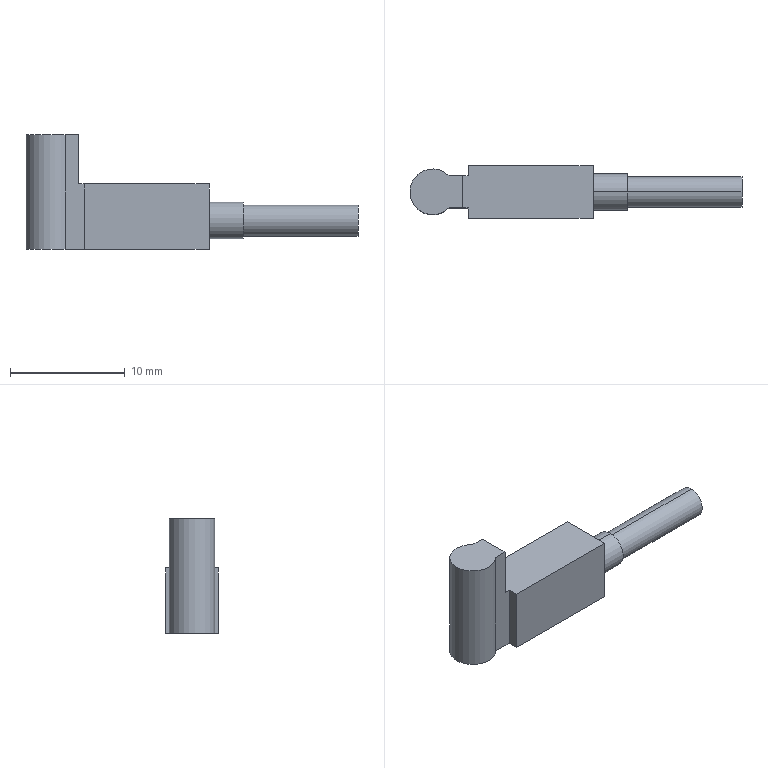Part | SolidWorks | features BaseBody 1 | 1 solid | 28 faces | box 29 x 4.6 x 10 mm | volume 522.344 mm3 | plane 18 | cylinder 10 | commonest cylinder face diameters 2.1 x3 2.5 x2 2.7 x2 3.2 x2 4 x1
STEP:
#1=CARTESIAN_POINT('',(27.,0.,-8.85));
#2=VERTEX_POINT('',#1);
#3=CARTESIAN_POINT('',(27.,0.,-6.15));
#4=VERTEX_POINT('',#3);
#5=CARTESIAN_POINT('',(27.,0.,-7.5));
#6=DIRECTION('',(1.,0.,0.));
#7=DIRECTION('',(0.,0.,-1.));
#8=AXIS2_PLACEMENT_3D('',#5,#6,#7);
#9=CIRCLE('',#8,1.35);
#10=EDGE_CURVE('',#2,#4,#9,.T.);
#11=ORIENTED_EDGE('',*,*,#10,.F.);
#12=CARTESIAN_POINT('',(17.,0.,-8.85));
#13=VERTEX_POINT('',#12);
#14=CARTESIAN_POINT('',(27.,0.,-8.85));
#15=DIRECTION('',(-1.,0.,0.));
#16=VECTOR('',#15,1000.);
#17=LINE('',#14,#16);
#18=EDGE_CURVE('',#2,#13,#17,.T.);
#19=ORIENTED_EDGE('',*,*,#18,.T.);
#20=CARTESIAN_POINT('',(17.,0.,-6.15));
#21=VERTEX_POINT('',#20);
#22=CARTESIAN_POINT('',(17.,0.,-7.5));
#23=DIRECTION('',(-1.,0.,0.));
#24=DIRECTION('',(0.,0.,-1.));
#25=AXIS2_PLACEMENT_3D('',#22,#23,#24);
#26=CIRCLE('',#25,1.35);
#27=EDGE_CURVE('',#21,#13,#26,.T.);
#28=ORIENTED_EDGE('',*,*,#27,.F.);
#29=CARTESIAN_POINT('',(27.,0.,-6.15));
#30=DIRECTION('',(-1.,0.,0.));
#31=VECTOR('',#30,1000.);
#32=LINE('',#29,#31);
#33=EDGE_CURVE('',#4,#21,#32,.T.);
#34=ORIENTED_EDGE('',*,*,#33,.F.);
#35=EDGE_LOOP('',(#11,#19,#28,#34));
#36=FACE_OUTER_BOUND('',#35,.T.);
#37=CARTESIAN_POINT('',(27.,0.,-7.5));
#38=DIRECTION('',(-1.,0.,0.));
#39=DIRECTION('',(0.,0.,1.));
#40=AXIS2_PLACEMENT_3D('',#37,#38,#39);
#41=CYLINDRICAL_SURFACE('',#40,1.35);
#42=ADVANCED_FACE('',(#36),#41,.T.);
#43=CARTESIAN_POINT('',(2.5,-0.4994,-2.924));
#44=VERTEX_POINT('',#43);
#45=CARTESIAN_POINT('',(2.5,0.,-3.05));
#46=VERTEX_POINT('',#45);
#47=CARTESIAN_POINT('',(2.5,0.,-2.));
#48=DIRECTION('',(1.,0.,0.));
#49=DIRECTION('',(0.,-0.4756,-0.8797));
#50=AXIS2_PLACEMENT_3D('',#47,#48,#49);
#51=CIRCLE('',#50,1.05);
#52=EDGE_CURVE('',#44,#46,#51,.T.);
#53=ORIENTED_EDGE('',*,*,#52,.T.);
#54=CARTESIAN_POINT('',(2.6,0.,-3.05));
#55=VERTEX_POINT('',#54);
#56=CARTESIAN_POINT('',(2.5,0.,-3.05));
#57=DIRECTION('',(1.,0.,0.));
#58=VECTOR('',#57,1000.);
#59=LINE('',#56,#58);
#60=EDGE_CURVE('',#46,#55,#59,.T.);
#61=ORIENTED_EDGE('',*,*,#60,.T.);
#62=CARTESIAN_POINT('',(2.6,-0.4994,-2.924));
#63=VERTEX_POINT('',#62);
#64=CARTESIAN_POINT('',(2.6,0.,-2.));
#65=DIRECTION('',(1.,0.,0.));
#66=DIRECTION('',(0.,-0.4756,-0.8797));
#67=AXIS2_PLACEMENT_3D('',#64,#65,#66);
#68=CIRCLE('',#67,1.05);
#69=EDGE_CURVE('',#63,#55,#68,.T.);
#70=ORIENTED_EDGE('',*,*,#69,.F.);
#71=CARTESIAN_POINT('',(2.6,-0.4994,-2.924));
#72=DIRECTION('',(-1.,0.,0.));
#73=VECTOR('',#72,1000.);
#74=LINE('',#71,#73);
#75=EDGE_CURVE('',#63,#44,#74,.T.);
#76=ORIENTED_EDGE('',*,*,#75,.T.);
#77=EDGE_LOOP('',(#53,#61,#70,#76));
#78=FACE_OUTER_BOUND('',#77,.T.);
#79=CARTESIAN_POINT('',(2.5,0.,-2.));
#80=DIRECTION('',(1.,0.,0.));
#81=DIRECTION('',(0.,0.,-1.));
#82=AXIS2_PLACEMENT_3D('',#79,#80,#81);
#83=CYLINDRICAL_SURFACE('',#82,1.05);
#84=ADVANCED_FACE('',(#78),#83,.T.);
#85=CARTESIAN_POINT('',(17.,0.,-9.1));
#86=VERTEX_POINT('',#85);
#87=CARTESIAN_POINT('',(17.,0.,-5.9));
#88=VERTEX_POINT('',#87);
#89=CARTESIAN_POINT('',(17.,0.,-7.5));
#90=DIRECTION('',(1.,0.,0.));
#91=DIRECTION('',(0.,0.,-1.));
#92=AXIS2_PLACEMENT_3D('',#89,#90,#91);
#93=CIRCLE('',#92,1.6);
#94=EDGE_CURVE('',#86,#88,#93,.T.);
#95=ORIENTED_EDGE('',*,*,#94,.F.);
#96=CARTESIAN_POINT('',(14.,0.,-9.1));
#97=VERTEX_POINT('',#96);
#98=CARTESIAN_POINT('',(17.,0.,-9.1));
#99=DIRECTION('',(-1.,0.,0.));
#100=VECTOR('',#99,1000.);
#101=LINE('',#98,#100);
#102=EDGE_CURVE('',#86,#97,#101,.T.);
#103=ORIENTED_EDGE('',*,*,#102,.T.);
#104=CARTESIAN_POINT('',(14.,0.,-5.9));
#105=VERTEX_POINT('',#104);
#106=CARTESIAN_POINT('',(14.,0.,-7.5));
#107=DIRECTION('',(1.,0.,0.));
#108=DIRECTION('',(0.,0.,-1.));
#109=AXIS2_PLACEMENT_3D('',#106,#107,#108);
#110=CIRCLE('',#109,1.6);
#111=EDGE_CURVE('',#97,#105,#110,.T.);
#112=ORIENTED_EDGE('',*,*,#111,.T.);
#113=CARTESIAN_POINT('',(17.,0.,-5.9));
#114=DIRECTION('',(-1.,0.,0.));
#115=VECTOR('',#114,1000.);
#116=LINE('',#113,#115);
#117=EDGE_CURVE('',#88,#105,#116,.T.);
#118=ORIENTED_EDGE('',*,*,#117,.F.);
#119=EDGE_LOOP('',(#95,#103,#112,#118));
#120=FACE_OUTER_BOUND('',#119,.T.);
#121=CARTESIAN_POINT('',(17.,0.,-7.5));
#122=DIRECTION('',(-1.,0.,0.));
#123=DIRECTION('',(0.,0.,1.));
#124=AXIS2_PLACEMENT_3D('',#121,#122,#123);
#125=CYLINDRICAL_SURFACE('',#124,1.6);
#126=ADVANCED_FACE('',(#120),#125,.T.);
#127=CARTESIAN_POINT('',(2.5,0.,-0.75));
#128=VERTEX_POINT('',#127);
#129=CARTESIAN_POINT('',(2.5,0.,-3.25));
#130=VERTEX_POINT('',#129);
#131=CARTESIAN_POINT('',(2.5,0.,-2.));
#132=DIRECTION('',(1.,0.,0.));
#133=DIRECTION('',(0.,0.,-1.));
#134=AXIS2_PLACEMENT_3D('',#131,#132,#133);
#135=CIRCLE('',#134,1.25);
#136=EDGE_CURVE('',#128,#130,#135,.T.);
#137=ORIENTED_EDGE('',*,*,#136,.F.);
#138=CARTESIAN_POINT('',(2.6,0.,-0.75));
#139=VERTEX_POINT('',#138);
#140=CARTESIAN_POINT('',(2.5,0.,-0.75));
#141=DIRECTION('',(1.,0.,0.));
#142=VECTOR('',#141,1000.);
#143=LINE('',#140,#142);
#144=EDGE_CURVE('',#128,#139,#143,.T.);
#145=ORIENTED_EDGE('',*,*,#144,.T.);
#146=CARTESIAN_POINT('',(2.6,0.,-3.25));
#147=VERTEX_POINT('',#146);
#148=CARTESIAN_POINT('',(2.6,0.,-2.));
#149=DIRECTION('',(1.,0.,0.));
#150=DIRECTION('',(0.,0.,-1.));
#151=AXIS2_PLACEMENT_3D('',#148,#149,#150);
#152=CIRCLE('',#151,1.25);
#153=EDGE_CURVE('',#139,#147,#152,.T.);
#154=ORIENTED_EDGE('',*,*,#153,.T.);
#155=CARTESIAN_POINT('',(2.5,0.,-3.25));
#156=DIRECTION('',(1.,0.,0.));
#157=VECTOR('',#156,1000.);
#158=LINE('',#155,#157);
#159=EDGE_CURVE('',#130,#147,#158,.T.);
#160=ORIENTED_EDGE('',*,*,#159,.F.);
#161=EDGE_LOOP('',(#137,#145,#154,#160));
#162=FACE_OUTER_BOUND('',#161,.T.);
#163=CARTESIAN_POINT('',(2.5,0.,-2.));
#164=DIRECTION('',(1.,0.,0.));
#165=DIRECTION('',(0.,0.,-1.));
#166=AXIS2_PLACEMENT_3D('',#163,#164,#165);
#167=CYLINDRICAL_SURFACE('',#166,1.25);
#168=ADVANCED_FACE('',(#162),#167,.F.);
#169=CARTESIAN_POINT('',(2.6,1.4,0.));
#170=VERTEX_POINT('',#169);
#171=CARTESIAN_POINT('',(1.428,1.4,0.));
#172=VERTEX_POINT('',#171);
#173=CARTESIAN_POINT('',(2.6,1.4,0.));
#174=DIRECTION('',(-1.,0.,0.));
#175=VECTOR('',#174,1000.);
#176=LINE('',#173,#175);
#177=EDGE_CURVE('',#170,#172,#176,.T.);
#178=ORIENTED_EDGE('',*,*,#177,.F.);
#179=CARTESIAN_POINT('',(2.6,1.4,-4.3));
#180=VERTEX_POINT('',#179);
#181=CARTESIAN_POINT('',(2.6,1.4,-4.3));
#182=DIRECTION('',(0.,0.,1.));
#183=VECTOR('',#182,1000.);
#184=LINE('',#181,#183);
#185=EDGE_CURVE('',#180,#170,#184,.T.);
#186=ORIENTED_EDGE('',*,*,#185,.F.);
#187=CARTESIAN_POINT('',(3.1,1.4,-4.3));
#188=VERTEX_POINT('',#187);
#189=CARTESIAN_POINT('',(3.1,1.4,-4.3));
#190=DIRECTION('',(-1.,0.,0.));
#191=VECTOR('',#190,1000.);
#192=LINE('',#189,#191);
#193=EDGE_CURVE('',#188,#180,#192,.T.);
#194=ORIENTED_EDGE('',*,*,#193,.F.);
#195=CARTESIAN_POINT('',(3.1,1.4,-10.));
#196=VERTEX_POINT('',#195);
#197=CARTESIAN_POINT('',(3.1,1.4,-4.3));
#198=DIRECTION('',(0.,0.,-1.));
#199=VECTOR('',#198,1000.);
#200=LINE('',#197,#199);
#201=EDGE_CURVE('',#188,#196,#200,.T.);
#202=ORIENTED_EDGE('',*,*,#201,.T.);
#203=CARTESIAN_POINT('',(1.428,1.4,-10.));
#204=VERTEX_POINT('',#203);
#205=CARTESIAN_POINT('',(3.1,1.4,-10.));
#206=DIRECTION('',(-1.,0.,0.));
#207=VECTOR('',#206,1000.);
#208=LINE('',#205,#207);
#209=EDGE_CURVE('',#196,#204,#208,.T.);
#210=ORIENTED_EDGE('',*,*,#209,.T.);
#211=CARTESIAN_POINT('',(1.428,1.4,-10.));
#212=DIRECTION('',(0.,0.,1.));
#213=VECTOR('',#212,1000.);
#214=LINE('',#211,#213);
#215=EDGE_CURVE('',#204,#172,#214,.T.);
#216=ORIENTED_EDGE('',*,*,#215,.T.);
#217=EDGE_LOOP('',(#178,#186,#194,#202,#210,#216));
#218=FACE_OUTER_BOUND('',#217,.T.);
#219=CARTESIAN_POINT('',(2.6,1.4,-10.));
#220=DIRECTION('',(0.,1.,0.));
#221=DIRECTION('',(0.,0.,1.));
#222=AXIS2_PLACEMENT_3D('',#219,#220,#221);
#223=PLANE('',#222);
#224=ADVANCED_FACE('',(#218),#223,.T.);
#225=ORIENTED_EDGE('',*,*,#177,.T.);
#226=CARTESIAN_POINT('',(1.428,-1.4,0.));
#227=VERTEX_POINT('',#226);
#228=CARTESIAN_POINT('',(0.,0.,0.));
#229=DIRECTION('',(0.,0.,1.));
#230=DIRECTION('',(0.7141,0.7,0.));
#231=AXIS2_PLACEMENT_3D('',#228,#229,#230);
#232=CIRCLE('',#231,2.);
#233=EDGE_CURVE('',#172,#227,#232,.T.);
#234=ORIENTED_EDGE('',*,*,#233,.T.);
#235=CARTESIAN_POINT('',(2.6,-1.4,0.));
#236=VERTEX_POINT('',#235);
#237=CARTESIAN_POINT('',(1.428,-1.4,0.));
#238=DIRECTION('',(1.,0.,0.));
#239=VECTOR('',#238,1000.);
#240=LINE('',#237,#239);
#241=EDGE_CURVE('',#227,#236,#240,.T.);
#242=ORIENTED_EDGE('',*,*,#241,.T.);
#243=CARTESIAN_POINT('',(2.6,-1.4,0.));
#244=DIRECTION('',(0.,1.,0.));
#245=VECTOR('',#244,1000.);
#246=LINE('',#243,#245);
#247=EDGE_CURVE('',#236,#170,#246,.T.);
#248=ORIENTED_EDGE('',*,*,#247,.T.);
#249=EDGE_LOOP('',(#225,#234,#242,#248));
#250=FACE_OUTER_BOUND('',#249,.T.);
#251=CARTESIAN_POINT('',(0.,0.,0.));
#252=DIRECTION('',(0.,0.,1.));
#253=DIRECTION('',(1.,0.,0.));
#254=AXIS2_PLACEMENT_3D('',#251,#252,#253);
#255=PLANE('',#254);
#256=ADVANCED_FACE('',(#250),#255,.T.);
#257=CARTESIAN_POINT('',(2.6,-1.4,-4.3));
#258=VERTEX_POINT('',#257);
#259=CARTESIAN_POINT('',(2.6,1.4,-4.3));
#260=DIRECTION('',(0.,-1.,0.));
#261=VECTOR('',#260,1000.);
#262=LINE('',#259,#261);
#263=EDGE_CURVE('',#180,#258,#262,.T.);
#264=ORIENTED_EDGE('',*,*,#263,.F.);
#265=ORIENTED_EDGE('',*,*,#185,.T.);
#266=ORIENTED_EDGE('',*,*,#247,.F.);
#267=CARTESIAN_POINT('',(2.6,-1.4,-4.3));
#268=DIRECTION('',(0.,0.,1.));
#269=VECTOR('',#268,1000.);
#270=LINE('',#267,#269);
#271=EDGE_CURVE('',#258,#236,#270,.T.);
#272=ORIENTED_EDGE('',*,*,#271,.F.);
#273=EDGE_LOOP('',(#264,#265,#266,#272));
#274=FACE_OUTER_BOUND('',#273,.T.);
#275=CARTESIAN_POINT('',(2.6,0.,-2.));
#276=DIRECTION('',(1.,0.,0.));
#277=DIRECTION('',(0.,0.,-1.));
#278=AXIS2_PLACEMENT_3D('',#275,#276,#277);
#279=CIRCLE('',#278,1.25);
#280=EDGE_CURVE('',#147,#139,#279,.T.);
#281=ORIENTED_EDGE('',*,*,#280,.F.);
#282=ORIENTED_EDGE('',*,*,#153,.F.);
#283=EDGE_LOOP('',(#281,#282));
#284=FACE_BOUND('',#283,.T.);
#285=CARTESIAN_POINT('',(2.6,-1.4,-10.));
#286=DIRECTION('',(1.,0.,0.));
#287=DIRECTION('',(0.,0.,-1.));
#288=AXIS2_PLACEMENT_3D('',#285,#286,#287);
#289=PLANE('',#288);
#290=ADVANCED_FACE('',(#274,#284),#289,.T.);
#291=ORIENTED_EDGE('',*,*,#193,.T.);
#292=ORIENTED_EDGE('',*,*,#263,.T.);
#293=CARTESIAN_POINT('',(3.1,-1.4,-4.3));
#294=VERTEX_POINT('',#293);
#295=CARTESIAN_POINT('',(2.6,-1.4,-4.3));
#296=DIRECTION('',(1.,0.,0.));
#297=VECTOR('',#296,1000.);
#298=LINE('',#295,#297);
#299=EDGE_CURVE('',#258,#294,#298,.T.);
#300=ORIENTED_EDGE('',*,*,#299,.T.);
#301=CARTESIAN_POINT('',(3.1,-2.3,-4.3));
#302=VERTEX_POINT('',#301);
#303=CARTESIAN_POINT('',(3.1,-1.4,-4.3));
#304=DIRECTION('',(0.,-1.,0.));
#305=VECTOR('',#304,1000.);
#306=LINE('',#303,#305);
#307=EDGE_CURVE('',#294,#302,#306,.T.);
#308=ORIENTED_EDGE('',*,*,#307,.T.);
#309=CARTESIAN_POINT('',(14.,-2.3,-4.3));
#310=VERTEX_POINT('',#309);
#311=CARTESIAN_POINT('',(3.1,-2.3,-4.3));
#312=DIRECTION('',(1.,0.,0.));
#313=VECTOR('',#312,1000.);
#314=LINE('',#311,#313);
#315=EDGE_CURVE('',#302,#310,#314,.T.);
#316=ORIENTED_EDGE('',*,*,#315,.T.);
#317=CARTESIAN_POINT('',(14.,2.3,-4.3));
#318=VERTEX_POINT('',#317);
#319=CARTESIAN_POINT('',(14.,-2.3,-4.3));
#320=DIRECTION('',(0.,1.,0.));
#321=VECTOR('',#320,1000.);
#322=LINE('',#319,#321);
#323=EDGE_CURVE('',#310,#318,#322,.T.);
#324=ORIENTED_EDGE('',*,*,#323,.T.);
#325=CARTESIAN_POINT('',(3.1,2.3,-4.3));
#326=VERTEX_POINT('',#325);
#327=CARTESIAN_POINT('',(14.,2.3,-4.3));
#328=DIRECTION('',(-1.,0.,0.));
#329=VECTOR('',#328,1000.);
#330=LINE('',#327,#329);
#331=EDGE_CURVE('',#318,#326,#330,.T.);
#332=ORIENTED_EDGE('',*,*,#331,.T.);
#333=CARTESIAN_POINT('',(3.1,2.3,-4.3));
#334=DIRECTION('',(0.,-1.,0.));
#335=VECTOR('',#334,1000.);
#336=LINE('',#333,#335);
#337=EDGE_CURVE('',#326,#188,#336,.T.);
#338=ORIENTED_EDGE('',*,*,#337,.T.);
#339=EDGE_LOOP('',(#291,#292,#300,#308,#316,#324,#332,#338));
#340=FACE_OUTER_BOUND('',#339,.T.);
#341=CARTESIAN_POINT('',(0.,0.,-4.3));
#342=DIRECTION('',(0.,0.,1.));
#343=DIRECTION('',(1.,0.,0.));
#344=AXIS2_PLACEMENT_3D('',#341,#342,#343);
#345=PLANE('',#344);
#346=ADVANCED_FACE('',(#340),#345,.T.);
#347=CARTESIAN_POINT('',(3.1,2.3,-10.));
#348=VERTEX_POINT('',#347);
#349=CARTESIAN_POINT('',(3.1,2.3,-10.));
#350=DIRECTION('',(0.,-1.,0.));
#351=VECTOR('',#350,1000.);
#352=LINE('',#349,#351);
#353=EDGE_CURVE('',#348,#196,#352,.T.);
#354=ORIENTED_EDGE('',*,*,#353,.T.);
#355=ORIENTED_EDGE('',*,*,#201,.F.);
#356=ORIENTED_EDGE('',*,*,#337,.F.);
#357=CARTESIAN_POINT('',(3.1,2.3,-4.3));
#358=DIRECTION('',(0.,0.,-1.));
#359=VECTOR('',#358,1000.);
#360=LINE('',#357,#359);
#361=EDGE_CURVE('',#326,#348,#360,.T.);
#362=ORIENTED_EDGE('',*,*,#361,.T.);
#363=EDGE_LOOP('',(#354,#355,#356,#362));
#364=FACE_OUTER_BOUND('',#363,.T.);
#365=CARTESIAN_POINT('',(3.1,2.3,-4.3));
#366=DIRECTION('',(1.,0.,0.));
#367=DIRECTION('',(0.,0.,-1.));
#368=AXIS2_PLACEMENT_3D('',#365,#366,#367);
#369=PLANE('',#368);
#370=ADVANCED_FACE('',(#364),#369,.F.);
#371=ORIENTED_EDGE('',*,*,#209,.F.);
#372=ORIENTED_EDGE('',*,*,#353,.F.);
#373=CARTESIAN_POINT('',(14.,2.3,-10.));
#374=VERTEX_POINT('',#373);
#375=CARTESIAN_POINT('',(14.,2.3,-10.));
#376=DIRECTION('',(-1.,0.,0.));
#377=VECTOR('',#376,1000.);
#378=LINE('',#375,#377);
#379=EDGE_CURVE('',#374,#348,#378,.T.);
#380=ORIENTED_EDGE('',*,*,#379,.F.);
#381=CARTESIAN_POINT('',(14.,-2.3,-10.));
#382=VERTEX_POINT('',#381);
#383=CARTESIAN_POINT('',(14.,-2.3,-10.));
#384=DIRECTION('',(0.,1.,0.));
#385=VECTOR('',#384,1000.);
#386=LINE('',#383,#385);
#387=EDGE_CURVE('',#382,#374,#386,.T.);
#388=ORIENTED_EDGE('',*,*,#387,.F.);
#389=CARTESIAN_POINT('',(3.1,-2.3,-10.));
#390=VERTEX_POINT('',#389);
#391=CARTESIAN_POINT('',(3.1,-2.3,-10.));
#392=DIRECTION('',(1.,0.,0.));
#393=VECTOR('',#392,1000.);
#394=LINE('',#391,#393);
#395=EDGE_CURVE('',#390,#382,#394,.T.);
#396=ORIENTED_EDGE('',*,*,#395,.F.);
#397=CARTESIAN_POINT('',(3.1,-1.4,-10.));
#398=VERTEX_POINT('',#397);
#399=CARTESIAN_POINT('',(3.1,-1.4,-10.));
#400=DIRECTION('',(0.,-1.,0.));
#401=VECTOR('',#400,1000.);
#402=LINE('',#399,#401);
#403=EDGE_CURVE('',#398,#390,#402,.T.);
#404=ORIENTED_EDGE('',*,*,#403,.F.);
#405=CARTESIAN_POINT('',(1.428,-1.4,-10.));
#406=VERTEX_POINT('',#405);
#407=CARTESIAN_POINT('',(1.428,-1.4,-10.));
#408=DIRECTION('',(1.,0.,0.));
#409=VECTOR('',#408,1000.);
#410=LINE('',#407,#409);
#411=EDGE_CURVE('',#406,#398,#410,.T.);
#412=ORIENTED_EDGE('',*,*,#411,.F.);
#413=CARTESIAN_POINT('',(0.,0.,-10.));
#414=DIRECTION('',(0.,0.,1.));
#415=DIRECTION('',(0.7141,0.7,0.));
#416=AXIS2_PLACEMENT_3D('',#413,#414,#415);
#417=CIRCLE('',#416,2.);
#418=EDGE_CURVE('',#204,#406,#417,.T.);
#419=ORIENTED_EDGE('',*,*,#418,.F.);
#420=EDGE_LOOP('',(#371,#372,#380,#388,#396,#404,#412,#419));
#421=FACE_OUTER_BOUND('',#420,.T.);
#422=CARTESIAN_POINT('',(0.,0.,-10.));
#423=DIRECTION('',(0.,0.,1.));
#424=DIRECTION('',(1.,0.,0.));
#425=AXIS2_PLACEMENT_3D('',#422,#423,#424);
#426=PLANE('',#425);
#427=ADVANCED_FACE('',(#421),#426,.F.);
#428=ORIENTED_EDGE('',*,*,#233,.F.);
#429=ORIENTED_EDGE('',*,*,#215,.F.);
#430=ORIENTED_EDGE('',*,*,#418,.T.);
#431=CARTESIAN_POINT('',(1.428,-1.4,-10.));
#432=DIRECTION('',(0.,0.,1.));
#433=VECTOR('',#432,1000.);
#434=LINE('',#431,#433);
#435=EDGE_CURVE('',#406,#227,#434,.T.);
#436=ORIENTED_EDGE('',*,*,#435,.T.);
#437=EDGE_LOOP('',(#428,#429,#430,#436));
#438=FACE_OUTER_BOUND('',#437,.T.);
#439=CARTESIAN_POINT('',(0.,0.,-10.));
#440=DIRECTION('',(0.,0.,1.));
#441=DIRECTION('',(1.,0.,0.));
#442=AXIS2_PLACEMENT_3D('',#439,#440,#441);
#443=CYLINDRICAL_SURFACE('',#442,2.);
#444=ADVANCED_FACE('',(#438),#443,.T.);
#445=ORIENTED_EDGE('',*,*,#241,.F.);
#446=ORIENTED_EDGE('',*,*,#435,.F.);
#447=ORIENTED_EDGE('',*,*,#411,.T.);
#448=CARTESIAN_POINT('',(3.1,-1.4,-4.3));
#449=DIRECTION('',(0.,0.,-1.));
#450=VECTOR('',#449,1000.);
#451=LINE('',#448,#450);
#452=EDGE_CURVE('',#294,#398,#451,.T.);
#453=ORIENTED_EDGE('',*,*,#452,.F.);
#454=ORIENTED_EDGE('',*,*,#299,.F.);
#455=ORIENTED_EDGE('',*,*,#271,.T.);
#456=EDGE_LOOP('',(#445,#446,#447,#453,#454,#455));
#457=FACE_OUTER_BOUND('',#456,.T.);
#458=CARTESIAN_POINT('',(1.428,-1.4,-10.));
#459=DIRECTION('',(0.,-1.,0.));
#460=DIRECTION('',(0.,0.,-1.));
#461=AXIS2_PLACEMENT_3D('',#458,#459,#460);
#462=PLANE('',#461);
#463=ADVANCED_FACE('',(#457),#462,.T.);
#464=ORIENTED_EDGE('',*,*,#144,.F.);
#465=CARTESIAN_POINT('',(2.5,0.,-2.));
#466=DIRECTION('',(1.,0.,0.));
#467=DIRECTION('',(0.,0.,-1.));
#468=AXIS2_PLACEMENT_3D('',#465,#466,#467);
#469=CIRCLE('',#468,1.25);
#470=EDGE_CURVE('',#130,#128,#469,.T.);
#471=ORIENTED_EDGE('',*,*,#470,.F.);
#472=ORIENTED_EDGE('',*,*,#159,.T.);
#473=ORIENTED_EDGE('',*,*,#280,.T.);
#474=EDGE_LOOP('',(#464,#471,#472,#473));
#475=FACE_OUTER_BOUND('',#474,.T.);
#476=CARTESIAN_POINT('',(2.5,0.,-2.));
#477=DIRECTION('',(1.,0.,0.));
#478=DIRECTION('',(0.,0.,-1.));
#479=AXIS2_PLACEMENT_3D('',#476,#477,#478);
#480=CYLINDRICAL_SURFACE('',#479,1.25);
#481=ADVANCED_FACE('',(#475),#480,.F.);
#482=ORIENTED_EDGE('',*,*,#403,.T.);
#483=CARTESIAN_POINT('',(3.1,-2.3,-4.3));
#484=DIRECTION('',(0.,0.,-1.));
#485=VECTOR('',#484,1000.);
#486=LINE('',#483,#485);
#487=EDGE_CURVE('',#302,#390,#486,.T.);
#488=ORIENTED_EDGE('',*,*,#487,.F.);
#489=ORIENTED_EDGE('',*,*,#307,.F.);
#490=ORIENTED_EDGE('',*,*,#452,.T.);
#491=EDGE_LOOP('',(#482,#488,#489,#490));
#492=FACE_OUTER_BOUND('',#491,.T.);
#493=CARTESIAN_POINT('',(3.1,-1.4,-4.3));
#494=DIRECTION('',(1.,0.,0.));
#495=DIRECTION('',(0.,0.,-1.));
#496=AXIS2_PLACEMENT_3D('',#493,#494,#495);
#497=PLANE('',#496);
#498=ADVANCED_FACE('',(#492),#497,.F.);
#499=ORIENTED_EDGE('',*,*,#395,.T.);
#500=CARTESIAN_POINT('',(14.,-2.3,-4.3));
#501=DIRECTION('',(0.,0.,-1.));
#502=VECTOR('',#501,1000.);
#503=LINE('',#500,#502);
#504=EDGE_CURVE('',#310,#382,#503,.T.);
#505=ORIENTED_EDGE('',*,*,#504,.F.);
#506=ORIENTED_EDGE('',*,*,#315,.F.);
#507=ORIENTED_EDGE('',*,*,#487,.T.);
#508=EDGE_LOOP('',(#499,#505,#506,#507));
#509=FACE_OUTER_BOUND('',#508,.T.);
#510=CARTESIAN_POINT('',(3.1,-2.3,-4.3));
#511=DIRECTION('',(0.,1.,0.));
#512=DIRECTION('',(0.,0.,1.));
#513=AXIS2_PLACEMENT_3D('',#510,#511,#512);
#514=PLANE('',#513);
#515=ADVANCED_FACE('',(#509),#514,.F.);
#516=CARTESIAN_POINT('',(14.,0.,-7.5));
#517=DIRECTION('',(1.,0.,0.));
#518=DIRECTION('',(0.,0.,-1.));
#519=AXIS2_PLACEMENT_3D('',#516,#517,#518);
#520=CIRCLE('',#519,1.6);
#521=EDGE_CURVE('',#105,#97,#520,.T.);
#522=ORIENTED_EDGE('',*,*,#521,.F.);
#523=ORIENTED_EDGE('',*,*,#111,.F.);
#524=EDGE_LOOP('',(#522,#523));
#525=FACE_BOUND('',#524,.T.);
#526=ORIENTED_EDGE('',*,*,#387,.T.);
#527=CARTESIAN_POINT('',(14.,2.3,-4.3));
#528=DIRECTION('',(0.,0.,-1.));
#529=VECTOR('',#528,1000.);
#530=LINE('',#527,#529);
#531=EDGE_CURVE('',#318,#374,#530,.T.);
#532=ORIENTED_EDGE('',*,*,#531,.F.);
#533=ORIENTED_EDGE('',*,*,#323,.F.);
#534=ORIENTED_EDGE('',*,*,#504,.T.);
#535=EDGE_LOOP('',(#526,#532,#533,#534));
#536=FACE_OUTER_BOUND('',#535,.T.);
#537=CARTESIAN_POINT('',(14.,-2.3,-4.3));
#538=DIRECTION('',(-1.,0.,0.));
#539=DIRECTION('',(0.,0.,1.));
#540=AXIS2_PLACEMENT_3D('',#537,#538,#539);
#541=PLANE('',#540);
#542=ADVANCED_FACE('',(#525,#536),#541,.F.);
#543=ORIENTED_EDGE('',*,*,#379,.T.);
#544=ORIENTED_EDGE('',*,*,#361,.F.);
#545=ORIENTED_EDGE('',*,*,#331,.F.);
#546=ORIENTED_EDGE('',*,*,#531,.T.);
#547=EDGE_LOOP('',(#543,#544,#545,#546));
#548=FACE_OUTER_BOUND('',#547,.T.);
#549=CARTESIAN_POINT('',(14.,2.3,-4.3));
#550=DIRECTION('',(0.,-1.,0.));
#551=DIRECTION('',(0.,0.,-1.));
#552=AXIS2_PLACEMENT_3D('',#549,#550,#551);
#553=PLANE('',#552);
#554=ADVANCED_FACE('',(#548),#553,.F.);
#555=CARTESIAN_POINT('',(2.5,0.4994,-1.076));
#556=VERTEX_POINT('',#555);
#557=CARTESIAN_POINT('',(2.5,-0.9236,-2.499));
#558=VERTEX_POINT('',#557);
#559=CARTESIAN_POINT('',(2.5,0.,-2.));
#560=DIRECTION('',(1.,0.,0.));
#561=DIRECTION('',(0.,0.4756,0.8797));
#562=AXIS2_PLACEMENT_3D('',#559,#560,#561);
#563=CIRCLE('',#562,1.05);
#564=EDGE_CURVE('',#556,#558,#563,.T.);
#565=ORIENTED_EDGE('',*,*,#564,.F.);
#566=CARTESIAN_POINT('',(2.5,0.4994,-1.076));
#567=DIRECTION('',(0.,-0.7071,-0.7071));
#568=VECTOR('',#567,1000.);
#569=LINE('',#566,#568);
#570=EDGE_CURVE('',#556,#558,#569,.T.);
#571=ORIENTED_EDGE('',*,*,#570,.T.);
#572=EDGE_LOOP('',(#565,#571));
#573=FACE_BOUND('',#572,.T.);
#574=CARTESIAN_POINT('',(2.5,0.9236,-1.501));
#575=VERTEX_POINT('',#574);
#576=CARTESIAN_POINT('',(2.5,-0.4994,-2.924));
#577=DIRECTION('',(0.,0.7071,0.7071));
#578=VECTOR('',#577,1000.);
#579=LINE('',#576,#578);
#580=EDGE_CURVE('',#44,#575,#579,.T.);
#581=ORIENTED_EDGE('',*,*,#580,.T.);
#582=CARTESIAN_POINT('',(2.5,0.,-2.));
#583=DIRECTION('',(1.,0.,0.));
#584=DIRECTION('',(0.,-0.4756,-0.8797));
#585=AXIS2_PLACEMENT_3D('',#582,#583,#584);
#586=CIRCLE('',#585,1.05);
#587=EDGE_CURVE('',#46,#575,#586,.T.);
#588=ORIENTED_EDGE('',*,*,#587,.F.);
#589=ORIENTED_EDGE('',*,*,#52,.F.);
#590=EDGE_LOOP('',(#581,#588,#589));
#591=FACE_BOUND('',#590,.T.);
#592=ORIENTED_EDGE('',*,*,#470,.T.);
#593=ORIENTED_EDGE('',*,*,#136,.T.);
#594=EDGE_LOOP('',(#592,#593));
#595=FACE_OUTER_BOUND('',#594,.T.);
#596=CARTESIAN_POINT('',(2.5,0.,-2.));
#597=DIRECTION('',(1.,0.,0.));
#598=DIRECTION('',(0.,0.,-1.));
#599=AXIS2_PLACEMENT_3D('',#596,#597,#598);
#600=PLANE('',#599);
#601=ADVANCED_FACE('',(#573,#591,#595),#600,.T.);
#602=ORIENTED_EDGE('',*,*,#102,.F.);
#603=CARTESIAN_POINT('',(17.,0.,-7.5));
#604=DIRECTION('',(1.,0.,0.));
#605=DIRECTION('',(0.,0.,-1.));
#606=AXIS2_PLACEMENT_3D('',#603,#604,#605);
#607=CIRCLE('',#606,1.6);
#608=EDGE_CURVE('',#88,#86,#607,.T.);
#609=ORIENTED_EDGE('',*,*,#608,.F.);
#610=ORIENTED_EDGE('',*,*,#117,.T.);
#611=ORIENTED_EDGE('',*,*,#521,.T.);
#612=EDGE_LOOP('',(#602,#609,#610,#611));
#613=FACE_OUTER_BOUND('',#612,.T.);
#614=CARTESIAN_POINT('',(17.,0.,-7.5));
#615=DIRECTION('',(-1.,0.,0.));
#616=DIRECTION('',(0.,0.,1.));
#617=AXIS2_PLACEMENT_3D('',#614,#615,#616);
#618=CYLINDRICAL_SURFACE('',#617,1.6);
#619=ADVANCED_FACE('',(#613),#618,.T.);
#620=CARTESIAN_POINT('',(2.6,-0.9236,-2.499));
#621=VERTEX_POINT('',#620);
#622=CARTESIAN_POINT('',(2.5,-0.9236,-2.499));
#623=DIRECTION('',(1.,0.,0.));
#624=VECTOR('',#623,1000.);
#625=LINE('',#622,#624);
#626=EDGE_CURVE('',#558,#621,#625,.T.);
#627=ORIENTED_EDGE('',*,*,#626,.T.);
#628=CARTESIAN_POINT('',(2.6,0.4994,-1.076));
#629=VERTEX_POINT('',#628);
#630=CARTESIAN_POINT('',(2.6,0.,-2.));
#631=DIRECTION('',(1.,0.,0.));
#632=DIRECTION('',(0.,0.4756,0.8797));
#633=AXIS2_PLACEMENT_3D('',#630,#631,#632);
#634=CIRCLE('',#633,1.05);
#635=EDGE_CURVE('',#629,#621,#634,.T.);
#636=ORIENTED_EDGE('',*,*,#635,.F.);
#637=CARTESIAN_POINT('',(2.6,0.4994,-1.076));
#638=DIRECTION('',(-1.,0.,0.));
#639=VECTOR('',#638,1000.);
#640=LINE('',#637,#639);
#641=EDGE_CURVE('',#629,#556,#640,.T.);
#642=ORIENTED_EDGE('',*,*,#641,.T.);
#643=ORIENTED_EDGE('',*,*,#564,.T.);
#644=EDGE_LOOP('',(#627,#636,#642,#643));
#645=FACE_OUTER_BOUND('',#644,.T.);
#646=CARTESIAN_POINT('',(2.5,0.,-2.));
#647=DIRECTION('',(1.,0.,0.));
#648=DIRECTION('',(0.,0.,-1.));
#649=AXIS2_PLACEMENT_3D('',#646,#647,#648);
#650=CYLINDRICAL_SURFACE('',#649,1.05);
#651=ADVANCED_FACE('',(#645),#650,.T.);
#652=ORIENTED_EDGE('',*,*,#626,.F.);
#653=ORIENTED_EDGE('',*,*,#570,.F.);
#654=ORIENTED_EDGE('',*,*,#641,.F.);
#655=CARTESIAN_POINT('',(2.6,0.4994,-1.076));
#656=DIRECTION('',(0.,-0.7071,-0.7071));
#657=VECTOR('',#656,1000.);
#658=LINE('',#655,#657);
#659=EDGE_CURVE('',#629,#621,#658,.T.);
#660=ORIENTED_EDGE('',*,*,#659,.T.);
#661=EDGE_LOOP('',(#652,#653,#654,#660));
#662=FACE_OUTER_BOUND('',#661,.T.);
#663=CARTESIAN_POINT('',(2.5,0.6095,-0.9663));
#664=DIRECTION('',(0.,-0.7071,0.7071));
#665=DIRECTION('',(0.,-0.7071,-0.7071));
#666=AXIS2_PLACEMENT_3D('',#663,#664,#665);
#667=PLANE('',#666);
#668=ADVANCED_FACE('',(#662),#667,.F.);
#669=CARTESIAN_POINT('',(2.6,0.9236,-1.501));
#670=VERTEX_POINT('',#669);
#671=CARTESIAN_POINT('',(2.5,0.9236,-1.501));
#672=DIRECTION('',(1.,0.,0.));
#673=VECTOR('',#672,1000.);
#674=LINE('',#671,#673);
#675=EDGE_CURVE('',#575,#670,#674,.T.);
#676=ORIENTED_EDGE('',*,*,#675,.F.);
#677=ORIENTED_EDGE('',*,*,#580,.F.);
#678=ORIENTED_EDGE('',*,*,#75,.F.);
#679=CARTESIAN_POINT('',(2.6,-0.4994,-2.924));
#680=DIRECTION('',(0.,0.7071,0.7071));
#681=VECTOR('',#680,1000.);
#682=LINE('',#679,#681);
#683=EDGE_CURVE('',#63,#670,#682,.T.);
#684=ORIENTED_EDGE('',*,*,#683,.T.);
#685=EDGE_LOOP('',(#676,#677,#678,#684));
#686=FACE_OUTER_BOUND('',#685,.T.);
#687=CARTESIAN_POINT('',(2.5,-0.6095,-3.034));
#688=DIRECTION('',(0.,0.7071,-0.7071));
#689=DIRECTION('',(0.,0.7071,0.7071));
#690=AXIS2_PLACEMENT_3D('',#687,#688,#689);
#691=PLANE('',#690);
#692=ADVANCED_FACE('',(#686),#691,.F.);
#693=ORIENTED_EDGE('',*,*,#60,.F.);
#694=ORIENTED_EDGE('',*,*,#587,.T.);
#695=ORIENTED_EDGE('',*,*,#675,.T.);
#696=CARTESIAN_POINT('',(2.6,0.,-2.));
#697=DIRECTION('',(1.,0.,0.));
#698=DIRECTION('',(0.,-0.4756,-0.8797));
#699=AXIS2_PLACEMENT_3D('',#696,#697,#698);
#700=CIRCLE('',#699,1.05);
#701=EDGE_CURVE('',#55,#670,#700,.T.);
#702=ORIENTED_EDGE('',*,*,#701,.F.);
#703=EDGE_LOOP('',(#693,#694,#695,#702));
#704=FACE_OUTER_BOUND('',#703,.T.);
#705=CARTESIAN_POINT('',(2.5,0.,-2.));
#706=DIRECTION('',(1.,0.,0.));
#707=DIRECTION('',(0.,0.,-1.));
#708=AXIS2_PLACEMENT_3D('',#705,#706,#707);
#709=CYLINDRICAL_SURFACE('',#708,1.05);
#710=ADVANCED_FACE('',(#704),#709,.T.);
#711=ORIENTED_EDGE('',*,*,#27,.T.);
#712=CARTESIAN_POINT('',(17.,0.,-7.5));
#713=DIRECTION('',(-1.,0.,0.));
#714=DIRECTION('',(0.,0.,-1.));
#715=AXIS2_PLACEMENT_3D('',#712,#713,#714);
#716=CIRCLE('',#715,1.35);
#717=EDGE_CURVE('',#13,#21,#716,.T.);
#718=ORIENTED_EDGE('',*,*,#717,.T.);
#719=EDGE_LOOP('',(#711,#718));
#720=FACE_BOUND('',#719,.T.);
#721=ORIENTED_EDGE('',*,*,#608,.T.);
#722=ORIENTED_EDGE('',*,*,#94,.T.);
#723=EDGE_LOOP('',(#721,#722));
#724=FACE_OUTER_BOUND('',#723,.T.);
#725=CARTESIAN_POINT('',(17.,0.,-7.5));
#726=DIRECTION('',(1.,0.,0.));
#727=DIRECTION('',(0.,0.,-1.));
#728=AXIS2_PLACEMENT_3D('',#725,#726,#727);
#729=PLANE('',#728);
#730=ADVANCED_FACE('',(#720,#724),#729,.T.);
#731=ORIENTED_EDGE('',*,*,#659,.F.);
#732=ORIENTED_EDGE('',*,*,#635,.T.);
#733=EDGE_LOOP('',(#731,#732));
#734=FACE_OUTER_BOUND('',#733,.T.);
#735=CARTESIAN_POINT('',(2.6,-1.4,-10.));
#736=DIRECTION('',(1.,0.,0.));
#737=DIRECTION('',(0.,0.,-1.));
#738=AXIS2_PLACEMENT_3D('',#735,#736,#737);
#739=PLANE('',#738);
#740=ADVANCED_FACE('',(#734),#739,.T.);
#741=ORIENTED_EDGE('',*,*,#683,.F.);
#742=ORIENTED_EDGE('',*,*,#69,.T.);
#743=ORIENTED_EDGE('',*,*,#701,.T.);
#744=EDGE_LOOP('',(#741,#742,#743));
#745=FACE_OUTER_BOUND('',#744,.T.);
#746=CARTESIAN_POINT('',(2.6,-1.4,-10.));
#747=DIRECTION('',(1.,0.,0.));
#748=DIRECTION('',(0.,0.,-1.));
#749=AXIS2_PLACEMENT_3D('',#746,#747,#748);
#750=PLANE('',#749);
#751=ADVANCED_FACE('',(#745),#750,.T.);
#752=ORIENTED_EDGE('',*,*,#18,.F.);
#753=CARTESIAN_POINT('',(27.,0.,-7.5));
#754=DIRECTION('',(1.,0.,0.));
#755=DIRECTION('',(0.,0.,-1.));
#756=AXIS2_PLACEMENT_3D('',#753,#754,#755);
#757=CIRCLE('',#756,1.35);
#758=EDGE_CURVE('',#4,#2,#757,.T.);
#759=ORIENTED_EDGE('',*,*,#758,.F.);
#760=ORIENTED_EDGE('',*,*,#33,.T.);
#761=ORIENTED_EDGE('',*,*,#717,.F.);
#762=EDGE_LOOP('',(#752,#759,#760,#761));
#763=FACE_OUTER_BOUND('',#762,.T.);
#764=CARTESIAN_POINT('',(27.,0.,-7.5));
#765=DIRECTION('',(-1.,0.,0.));
#766=DIRECTION('',(0.,0.,1.));
#767=AXIS2_PLACEMENT_3D('',#764,#765,#766);
#768=CYLINDRICAL_SURFACE('',#767,1.35);
#769=ADVANCED_FACE('',(#763),#768,.T.);
#770=ORIENTED_EDGE('',*,*,#758,.T.);
#771=ORIENTED_EDGE('',*,*,#10,.T.);
#772=EDGE_LOOP('',(#770,#771));
#773=FACE_OUTER_BOUND('',#772,.T.);
#774=CARTESIAN_POINT('',(27.,0.,-7.5));
#775=DIRECTION('',(1.,0.,0.));
#776=DIRECTION('',(0.,0.,-1.));
#777=AXIS2_PLACEMENT_3D('',#774,#775,#776);
#778=PLANE('',#777);
#779=ADVANCED_FACE('',(#773),#778,.T.);
#780=CLOSED_SHELL('',(#42,#84,#126,#168,#224,#256,#290,#346,#370,#427,#444,#463,#481,#498,#515,#542,#554,#601,#619,#651,#668,#692,#710,#730,#740,#751,#769,#779));
#781=MANIFOLD_SOLID_BREP('',#780);
#782=CARTESIAN_POINT('',(0.,0.,0.));
#783=DIRECTION('',(0.,0.,1.));
#784=DIRECTION('',(1.,0.,0.));
#785=AXIS2_PLACEMENT_3D('',#782,#783,#784);
#786=(LENGTH_UNIT()NAMED_UNIT(*)SI_UNIT(.MILLI.,.METRE.));
#787=UNCERTAINTY_MEASURE_WITH_UNIT(LENGTH_MEASURE(0.00001),#786,'','');
#788=(NAMED_UNIT(*)PLANE_ANGLE_UNIT()SI_UNIT($,.RADIAN.));
#789=(NAMED_UNIT(*)SI_UNIT($,.STERADIAN.)SOLID_ANGLE_UNIT());
#790=(GEOMETRIC_REPRESENTATION_CONTEXT(3)GLOBAL_UNCERTAINTY_ASSIGNED_CONTEXT((#787))GLOBAL_UNIT_ASSIGNED_CONTEXT((#786,#788,#789))REPRESENTATION_CONTEXT('',''));
#791=ADVANCED_BREP_SHAPE_REPRESENTATION('',(#781,#785),#790);